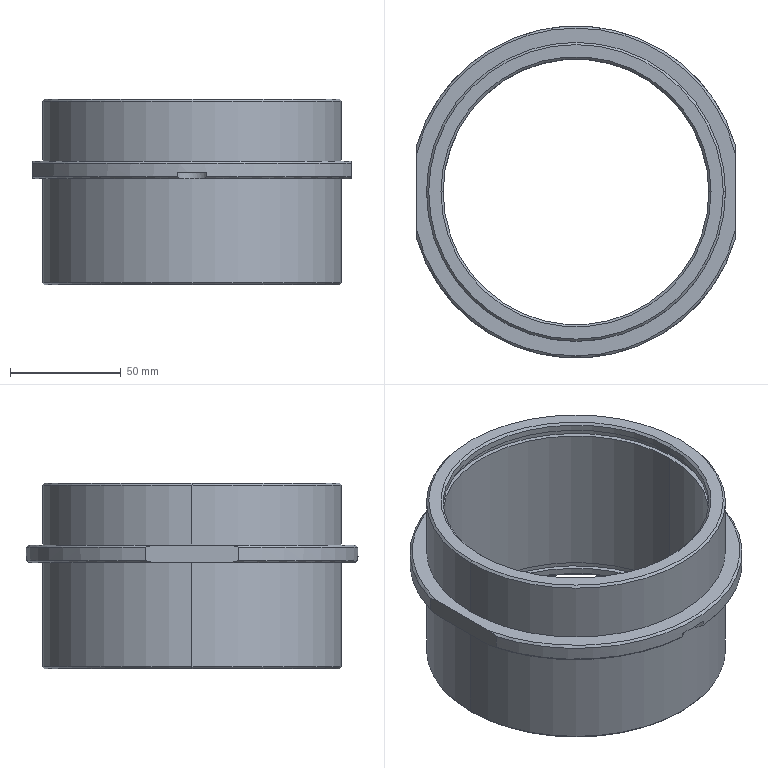Part | SolidWorks | features ICE 4, Chamfer 1, Extrusion 1, RevCut 1 | 1 solid | 44 faces | box 144 x 150 x 84 mm | volume 271588 mm3 | cylinder 18 | cone 14 | plane 12 | commonest cylinder face diameters 120 x6 124 x4 135 x4 16 x2 150 x2
STEP:
#1=CARTESIAN_POINT('',(66.5,0.,36.));
#2=VERTEX_POINT('',#1);
#3=CARTESIAN_POINT('',(-66.5,0.,36.));
#4=VERTEX_POINT('',#3);
#5=CARTESIAN_POINT('',(0.,0.,36.));
#6=DIRECTION('',(0.,0.,1.));
#7=DIRECTION('',(1.,0.,0.));
#8=AXIS2_PLACEMENT_3D('',#5,#6,#7);
#9=CIRCLE('',#8,66.5);
#10=EDGE_CURVE('',#2,#4,#9,.T.);
#11=ORIENTED_EDGE('',*,*,#10,.F.);
#12=CARTESIAN_POINT('',(67.5,0.,35.));
#13=VERTEX_POINT('',#12);
#14=CARTESIAN_POINT('',(66.5,0.,36.));
#15=DIRECTION('',(0.7071,0.,-0.7071));
#16=VECTOR('',#15,1000.);
#17=LINE('',#14,#16);
#18=EDGE_CURVE('',#2,#13,#17,.T.);
#19=ORIENTED_EDGE('',*,*,#18,.T.);
#20=CARTESIAN_POINT('',(-67.5,0.,35.));
#21=VERTEX_POINT('',#20);
#22=CARTESIAN_POINT('',(0.,0.,35.));
#23=DIRECTION('',(0.,0.,-1.));
#24=DIRECTION('',(1.,0.,0.));
#25=AXIS2_PLACEMENT_3D('',#22,#23,#24);
#26=CIRCLE('',#25,67.5);
#27=EDGE_CURVE('',#21,#13,#26,.T.);
#28=ORIENTED_EDGE('',*,*,#27,.F.);
#29=CARTESIAN_POINT('',(-66.5,0.,36.));
#30=DIRECTION('',(-0.7071,0.,-0.7071));
#31=VECTOR('',#30,1000.);
#32=LINE('',#29,#31);
#33=EDGE_CURVE('',#4,#21,#32,.T.);
#34=ORIENTED_EDGE('',*,*,#33,.F.);
#35=EDGE_LOOP('',(#11,#19,#28,#34));
#36=FACE_OUTER_BOUND('',#35,.T.);
#37=CARTESIAN_POINT('',(0.,0.,36.));
#38=DIRECTION('',(0.,0.,-1.));
#39=DIRECTION('',(-1.,0.,0.));
#40=AXIS2_PLACEMENT_3D('',#37,#38,#39);
#41=CONICAL_SURFACE('',#40,66.5,0.7854);
#42=ADVANCED_FACE('',(#36),#41,.T.);
#43=CARTESIAN_POINT('',(-60.,0.,35.));
#44=VERTEX_POINT('',#43);
#45=CARTESIAN_POINT('',(60.,0.,35.));
#46=VERTEX_POINT('',#45);
#47=CARTESIAN_POINT('',(0.,0.,35.));
#48=DIRECTION('',(0.,0.,1.));
#49=DIRECTION('',(1.,0.,0.));
#50=AXIS2_PLACEMENT_3D('',#47,#48,#49);
#51=CIRCLE('',#50,60.);
#52=EDGE_CURVE('',#44,#46,#51,.T.);
#53=ORIENTED_EDGE('',*,*,#52,.F.);
#54=CARTESIAN_POINT('',(-61.,0.,36.));
#55=VERTEX_POINT('',#54);
#56=CARTESIAN_POINT('',(-60.,0.,35.));
#57=DIRECTION('',(-0.7071,0.,0.7071));
#58=VECTOR('',#57,1000.);
#59=LINE('',#56,#58);
#60=EDGE_CURVE('',#44,#55,#59,.T.);
#61=ORIENTED_EDGE('',*,*,#60,.T.);
#62=CARTESIAN_POINT('',(61.,0.,36.));
#63=VERTEX_POINT('',#62);
#64=CARTESIAN_POINT('',(0.,0.,36.));
#65=DIRECTION('',(0.,0.,-1.));
#66=DIRECTION('',(1.,0.,0.));
#67=AXIS2_PLACEMENT_3D('',#64,#65,#66);
#68=CIRCLE('',#67,61.);
#69=EDGE_CURVE('',#63,#55,#68,.T.);
#70=ORIENTED_EDGE('',*,*,#69,.F.);
#71=CARTESIAN_POINT('',(60.,0.,35.));
#72=DIRECTION('',(0.7071,0.,0.7071));
#73=VECTOR('',#72,1000.);
#74=LINE('',#71,#73);
#75=EDGE_CURVE('',#46,#63,#74,.T.);
#76=ORIENTED_EDGE('',*,*,#75,.F.);
#77=EDGE_LOOP('',(#53,#61,#70,#76));
#78=FACE_OUTER_BOUND('',#77,.T.);
#79=CARTESIAN_POINT('',(0.,0.,35.));
#80=DIRECTION('',(0.,0.,1.));
#81=DIRECTION('',(1.,0.,0.));
#82=AXIS2_PLACEMENT_3D('',#79,#80,#81);
#83=CONICAL_SURFACE('',#82,60.,0.7854);
#84=ADVANCED_FACE('',(#78),#83,.F.);
#85=CARTESIAN_POINT('',(60.,0.,-47.));
#86=VERTEX_POINT('',#85);
#87=CARTESIAN_POINT('',(-60.,0.,-47.));
#88=VERTEX_POINT('',#87);
#89=CARTESIAN_POINT('',(0.,0.,-47.));
#90=DIRECTION('',(0.,0.,-1.));
#91=DIRECTION('',(1.,0.,0.));
#92=AXIS2_PLACEMENT_3D('',#89,#90,#91);
#93=CIRCLE('',#92,60.);
#94=EDGE_CURVE('',#86,#88,#93,.T.);
#95=ORIENTED_EDGE('',*,*,#94,.F.);
#96=CARTESIAN_POINT('',(61.,0.,-48.));
#97=VERTEX_POINT('',#96);
#98=CARTESIAN_POINT('',(61.,0.,-48.));
#99=DIRECTION('',(0.7071,0.,-0.7071));
#100=VECTOR('',#99,1000.);
#101=LINE('',#98,#100);
#102=EDGE_CURVE('',#86,#97,#101,.T.);
#103=ORIENTED_EDGE('',*,*,#102,.T.);
#104=CARTESIAN_POINT('',(-61.,0.,-48.));
#105=VERTEX_POINT('',#104);
#106=CARTESIAN_POINT('',(0.,0.,-48.));
#107=DIRECTION('',(0.,0.,1.));
#108=DIRECTION('',(1.,0.,0.));
#109=AXIS2_PLACEMENT_3D('',#106,#107,#108);
#110=CIRCLE('',#109,61.);
#111=EDGE_CURVE('',#105,#97,#110,.T.);
#112=ORIENTED_EDGE('',*,*,#111,.F.);
#113=CARTESIAN_POINT('',(-61.,0.,-48.));
#114=DIRECTION('',(-0.7071,0.,-0.7071));
#115=VECTOR('',#114,1000.);
#116=LINE('',#113,#115);
#117=EDGE_CURVE('',#88,#105,#116,.T.);
#118=ORIENTED_EDGE('',*,*,#117,.F.);
#119=EDGE_LOOP('',(#95,#103,#112,#118));
#120=FACE_OUTER_BOUND('',#119,.T.);
#121=CARTESIAN_POINT('',(0.,0.,-48.));
#122=DIRECTION('',(0.,0.,-1.));
#123=DIRECTION('',(-1.,0.,0.));
#124=AXIS2_PLACEMENT_3D('',#121,#122,#123);
#125=CONICAL_SURFACE('',#124,61.,0.7854);
#126=ADVANCED_FACE('',(#120),#125,.F.);
#127=CARTESIAN_POINT('',(-66.5,0.,-48.));
#128=VERTEX_POINT('',#127);
#129=CARTESIAN_POINT('',(66.5,0.,-48.));
#130=VERTEX_POINT('',#129);
#131=CARTESIAN_POINT('',(0.,0.,-48.));
#132=DIRECTION('',(0.,0.,-1.));
#133=DIRECTION('',(1.,0.,0.));
#134=AXIS2_PLACEMENT_3D('',#131,#132,#133);
#135=CIRCLE('',#134,66.5);
#136=EDGE_CURVE('',#128,#130,#135,.T.);
#137=ORIENTED_EDGE('',*,*,#136,.F.);
#138=CARTESIAN_POINT('',(-67.5,0.,-47.));
#139=VERTEX_POINT('',#138);
#140=CARTESIAN_POINT('',(-67.5,0.,-47.));
#141=DIRECTION('',(-0.7071,0.,0.7071));
#142=VECTOR('',#141,1000.);
#143=LINE('',#140,#142);
#144=EDGE_CURVE('',#128,#139,#143,.T.);
#145=ORIENTED_EDGE('',*,*,#144,.T.);
#146=CARTESIAN_POINT('',(67.5,0.,-47.));
#147=VERTEX_POINT('',#146);
#148=CARTESIAN_POINT('',(0.,0.,-47.));
#149=DIRECTION('',(0.,0.,1.));
#150=DIRECTION('',(1.,0.,0.));
#151=AXIS2_PLACEMENT_3D('',#148,#149,#150);
#152=CIRCLE('',#151,67.5);
#153=EDGE_CURVE('',#147,#139,#152,.T.);
#154=ORIENTED_EDGE('',*,*,#153,.F.);
#155=CARTESIAN_POINT('',(67.5,0.,-47.));
#156=DIRECTION('',(0.7071,0.,0.7071));
#157=VECTOR('',#156,1000.);
#158=LINE('',#155,#157);
#159=EDGE_CURVE('',#130,#147,#158,.T.);
#160=ORIENTED_EDGE('',*,*,#159,.F.);
#161=EDGE_LOOP('',(#137,#145,#154,#160));
#162=FACE_OUTER_BOUND('',#161,.T.);
#163=CARTESIAN_POINT('',(0.,0.,-47.));
#164=DIRECTION('',(0.,0.,1.));
#165=DIRECTION('',(1.,0.,0.));
#166=AXIS2_PLACEMENT_3D('',#163,#164,#165);
#167=CONICAL_SURFACE('',#166,67.5,0.7854);
#168=ADVANCED_FACE('',(#162),#167,.T.);
#169=CARTESIAN_POINT('',(62.,0.,32.2));
#170=VERTEX_POINT('',#169);
#171=CARTESIAN_POINT('',(-62.,0.,32.2));
#172=VERTEX_POINT('',#171);
#173=CARTESIAN_POINT('',(0.,0.,32.2));
#174=DIRECTION('',(0.,0.,-1.));
#175=DIRECTION('',(-1.,0.,0.));
#176=AXIS2_PLACEMENT_3D('',#173,#174,#175);
#177=CIRCLE('',#176,62.);
#178=EDGE_CURVE('',#170,#172,#177,.T.);
#179=ORIENTED_EDGE('',*,*,#178,.F.);
#180=CARTESIAN_POINT('',(62.,0.,29.));
#181=VERTEX_POINT('',#180);
#182=CARTESIAN_POINT('',(62.,0.,-49.991));
#183=DIRECTION('',(0.,0.,-1.));
#184=VECTOR('',#183,1000.);
#185=LINE('',#182,#184);
#186=EDGE_CURVE('',#170,#181,#185,.T.);
#187=ORIENTED_EDGE('',*,*,#186,.T.);
#188=CARTESIAN_POINT('',(-62.,0.,29.));
#189=VERTEX_POINT('',#188);
#190=CARTESIAN_POINT('',(0.,0.,29.));
#191=DIRECTION('',(0.,0.,-1.));
#192=DIRECTION('',(-1.,0.,0.));
#193=AXIS2_PLACEMENT_3D('',#190,#191,#192);
#194=CIRCLE('',#193,62.);
#195=EDGE_CURVE('',#181,#189,#194,.T.);
#196=ORIENTED_EDGE('',*,*,#195,.T.);
#197=CARTESIAN_POINT('',(-62.,0.,-49.991));
#198=DIRECTION('',(0.,0.,-1.));
#199=VECTOR('',#198,1000.);
#200=LINE('',#197,#199);
#201=EDGE_CURVE('',#172,#189,#200,.T.);
#202=ORIENTED_EDGE('',*,*,#201,.F.);
#203=EDGE_LOOP('',(#179,#187,#196,#202));
#204=FACE_OUTER_BOUND('',#203,.T.);
#205=CARTESIAN_POINT('',(0.,0.,-49.991));
#206=DIRECTION('',(0.,0.,-1.));
#207=DIRECTION('',(-1.,0.,0.));
#208=AXIS2_PLACEMENT_3D('',#205,#206,#207);
#209=CYLINDRICAL_SURFACE('',#208,62.);
#210=ADVANCED_FACE('',(#204),#209,.F.);
#211=CARTESIAN_POINT('',(60.,0.,-41.));
#212=VERTEX_POINT('',#211);
#213=CARTESIAN_POINT('',(-60.,0.,-41.));
#214=VERTEX_POINT('',#213);
#215=CARTESIAN_POINT('',(0.,0.,-41.));
#216=DIRECTION('',(0.,0.,-1.));
#217=DIRECTION('',(1.,0.,0.));
#218=AXIS2_PLACEMENT_3D('',#215,#216,#217);
#219=CIRCLE('',#218,60.);
#220=EDGE_CURVE('',#212,#214,#219,.T.);
#221=ORIENTED_EDGE('',*,*,#220,.T.);
#222=CARTESIAN_POINT('',(-60.,0.,29.));
#223=VERTEX_POINT('',#222);
#224=CARTESIAN_POINT('',(-60.,0.,-124.));
#225=DIRECTION('',(0.,0.,1.));
#226=VECTOR('',#225,1000.);
#227=LINE('',#224,#226);
#228=EDGE_CURVE('',#214,#223,#227,.T.);
#229=ORIENTED_EDGE('',*,*,#228,.T.);
#230=CARTESIAN_POINT('',(60.,0.,29.));
#231=VERTEX_POINT('',#230);
#232=CARTESIAN_POINT('',(0.,0.,29.));
#233=DIRECTION('',(0.,0.,1.));
#234=DIRECTION('',(-1.,0.,0.));
#235=AXIS2_PLACEMENT_3D('',#232,#233,#234);
#236=CIRCLE('',#235,60.);
#237=EDGE_CURVE('',#223,#231,#236,.T.);
#238=ORIENTED_EDGE('',*,*,#237,.T.);
#239=CARTESIAN_POINT('',(60.,0.,-124.));
#240=DIRECTION('',(0.,0.,1.));
#241=VECTOR('',#240,1000.);
#242=LINE('',#239,#241);
#243=EDGE_CURVE('',#212,#231,#242,.T.);
#244=ORIENTED_EDGE('',*,*,#243,.F.);
#245=EDGE_LOOP('',(#221,#229,#238,#244));
#246=FACE_OUTER_BOUND('',#245,.T.);
#247=CARTESIAN_POINT('',(0.,0.,-124.));
#248=DIRECTION('',(0.,0.,1.));
#249=DIRECTION('',(1.,0.,0.));
#250=AXIS2_PLACEMENT_3D('',#247,#248,#249);
#251=CYLINDRICAL_SURFACE('',#250,60.);
#252=ADVANCED_FACE('',(#246),#251,.F.);
#253=CARTESIAN_POINT('',(62.,0.,-41.));
#254=VERTEX_POINT('',#253);
#255=CARTESIAN_POINT('',(-62.,0.,-41.));
#256=VERTEX_POINT('',#255);
#257=CARTESIAN_POINT('',(0.,0.,-41.));
#258=DIRECTION('',(0.,0.,-1.));
#259=DIRECTION('',(-1.,0.,0.));
#260=AXIS2_PLACEMENT_3D('',#257,#258,#259);
#261=CIRCLE('',#260,62.);
#262=EDGE_CURVE('',#254,#256,#261,.T.);
#263=ORIENTED_EDGE('',*,*,#262,.F.);
#264=CARTESIAN_POINT('',(62.,0.,-44.2));
#265=VERTEX_POINT('',#264);
#266=CARTESIAN_POINT('',(62.,0.,-49.991));
#267=DIRECTION('',(0.,0.,-1.));
#268=VECTOR('',#267,1000.);
#269=LINE('',#266,#268);
#270=EDGE_CURVE('',#254,#265,#269,.T.);
#271=ORIENTED_EDGE('',*,*,#270,.T.);
#272=CARTESIAN_POINT('',(-62.,0.,-44.2));
#273=VERTEX_POINT('',#272);
#274=CARTESIAN_POINT('',(0.,0.,-44.2));
#275=DIRECTION('',(0.,0.,-1.));
#276=DIRECTION('',(-1.,0.,0.));
#277=AXIS2_PLACEMENT_3D('',#274,#275,#276);
#278=CIRCLE('',#277,62.);
#279=EDGE_CURVE('',#265,#273,#278,.T.);
#280=ORIENTED_EDGE('',*,*,#279,.T.);
#281=CARTESIAN_POINT('',(-62.,0.,-49.991));
#282=DIRECTION('',(0.,0.,-1.));
#283=VECTOR('',#282,1000.);
#284=LINE('',#281,#283);
#285=EDGE_CURVE('',#256,#273,#284,.T.);
#286=ORIENTED_EDGE('',*,*,#285,.F.);
#287=EDGE_LOOP('',(#263,#271,#280,#286));
#288=FACE_OUTER_BOUND('',#287,.T.);
#289=CARTESIAN_POINT('',(0.,0.,-49.991));
#290=DIRECTION('',(0.,0.,-1.));
#291=DIRECTION('',(-1.,0.,0.));
#292=AXIS2_PLACEMENT_3D('',#289,#290,#291);
#293=CYLINDRICAL_SURFACE('',#292,62.);
#294=ADVANCED_FACE('',(#288),#293,.F.);
#295=ORIENTED_EDGE('',*,*,#94,.T.);
#296=CARTESIAN_POINT('',(-60.,0.,-44.2));
#297=VERTEX_POINT('',#296);
#298=CARTESIAN_POINT('',(-60.,0.,-124.));
#299=DIRECTION('',(0.,0.,1.));
#300=VECTOR('',#299,1000.);
#301=LINE('',#298,#300);
#302=EDGE_CURVE('',#88,#297,#301,.T.);
#303=ORIENTED_EDGE('',*,*,#302,.T.);
#304=CARTESIAN_POINT('',(60.,0.,-44.2));
#305=VERTEX_POINT('',#304);
#306=CARTESIAN_POINT('',(0.,0.,-44.2));
#307=DIRECTION('',(0.,0.,1.));
#308=DIRECTION('',(-1.,0.,0.));
#309=AXIS2_PLACEMENT_3D('',#306,#307,#308);
#310=CIRCLE('',#309,60.);
#311=EDGE_CURVE('',#297,#305,#310,.T.);
#312=ORIENTED_EDGE('',*,*,#311,.T.);
#313=CARTESIAN_POINT('',(60.,0.,-124.));
#314=DIRECTION('',(0.,0.,1.));
#315=VECTOR('',#314,1000.);
#316=LINE('',#313,#315);
#317=EDGE_CURVE('',#86,#305,#316,.T.);
#318=ORIENTED_EDGE('',*,*,#317,.F.);
#319=EDGE_LOOP('',(#295,#303,#312,#318));
#320=FACE_OUTER_BOUND('',#319,.T.);
#321=CARTESIAN_POINT('',(0.,0.,-124.));
#322=DIRECTION('',(0.,0.,1.));
#323=DIRECTION('',(1.,0.,0.));
#324=AXIS2_PLACEMENT_3D('',#321,#322,#323);
#325=CYLINDRICAL_SURFACE('',#324,60.);
#326=ADVANCED_FACE('',(#320),#325,.F.);
#327=CARTESIAN_POINT('',(67.5,0.,8.));
#328=VERTEX_POINT('',#327);
#329=CARTESIAN_POINT('',(-67.5,0.,8.));
#330=VERTEX_POINT('',#329);
#331=CARTESIAN_POINT('',(0.,0.,8.));
#332=DIRECTION('',(0.,0.,1.));
#333=DIRECTION('',(1.,0.,0.));
#334=AXIS2_PLACEMENT_3D('',#331,#332,#333);
#335=CIRCLE('',#334,67.5);
#336=EDGE_CURVE('',#328,#330,#335,.T.);
#337=ORIENTED_EDGE('',*,*,#336,.T.);
#338=CARTESIAN_POINT('',(-67.5,0.,-48.));
#339=DIRECTION('',(0.,0.,1.));
#340=VECTOR('',#339,1000.);
#341=LINE('',#338,#340);
#342=EDGE_CURVE('',#330,#21,#341,.T.);
#343=ORIENTED_EDGE('',*,*,#342,.T.);
#344=ORIENTED_EDGE('',*,*,#27,.T.);
#345=CARTESIAN_POINT('',(67.5,0.,-48.));
#346=DIRECTION('',(0.,0.,1.));
#347=VECTOR('',#346,1000.);
#348=LINE('',#345,#347);
#349=EDGE_CURVE('',#328,#13,#348,.T.);
#350=ORIENTED_EDGE('',*,*,#349,.F.);
#351=EDGE_LOOP('',(#337,#343,#344,#350));
#352=FACE_OUTER_BOUND('',#351,.T.);
#353=CARTESIAN_POINT('',(0.,0.,-48.));
#354=DIRECTION('',(0.,0.,1.));
#355=DIRECTION('',(1.,0.,0.));
#356=AXIS2_PLACEMENT_3D('',#353,#354,#355);
#357=CYLINDRICAL_SURFACE('',#356,67.5);
#358=ADVANCED_FACE('',(#352),#357,.T.);
#359=ORIENTED_EDGE('',*,*,#153,.T.);
#360=CARTESIAN_POINT('',(-67.5,0.,0.));
#361=VERTEX_POINT('',#360);
#362=CARTESIAN_POINT('',(-67.5,0.,-48.));
#363=DIRECTION('',(0.,0.,1.));
#364=VECTOR('',#363,1000.);
#365=LINE('',#362,#364);
#366=EDGE_CURVE('',#139,#361,#365,.T.);
#367=ORIENTED_EDGE('',*,*,#366,.T.);
#368=CARTESIAN_POINT('',(67.5,0.,0.));
#369=VERTEX_POINT('',#368);
#370=CARTESIAN_POINT('',(0.,0.,0.));
#371=DIRECTION('',(0.,0.,1.));
#372=DIRECTION('',(1.,0.,0.));
#373=AXIS2_PLACEMENT_3D('',#370,#371,#372);
#374=CIRCLE('',#373,67.5);
#375=EDGE_CURVE('',#369,#361,#374,.T.);
#376=ORIENTED_EDGE('',*,*,#375,.F.);
#377=CARTESIAN_POINT('',(67.5,0.,-48.));
#378=DIRECTION('',(0.,0.,1.));
#379=VECTOR('',#378,1000.);
#380=LINE('',#377,#379);
#381=EDGE_CURVE('',#147,#369,#380,.T.);
#382=ORIENTED_EDGE('',*,*,#381,.F.);
#383=EDGE_LOOP('',(#359,#367,#376,#382));
#384=FACE_OUTER_BOUND('',#383,.T.);
#385=CARTESIAN_POINT('',(0.,0.,-48.));
#386=DIRECTION('',(0.,0.,1.));
#387=DIRECTION('',(1.,0.,0.));
#388=AXIS2_PLACEMENT_3D('',#385,#386,#387);
#389=CYLINDRICAL_SURFACE('',#388,67.5);
#390=ADVANCED_FACE('',(#384),#389,.T.);
#391=CARTESIAN_POINT('',(60.,0.,32.2));
#392=VERTEX_POINT('',#391);
#393=CARTESIAN_POINT('',(-60.,0.,32.2));
#394=VERTEX_POINT('',#393);
#395=CARTESIAN_POINT('',(0.,0.,32.2));
#396=DIRECTION('',(0.,0.,-1.));
#397=DIRECTION('',(1.,0.,0.));
#398=AXIS2_PLACEMENT_3D('',#395,#396,#397);
#399=CIRCLE('',#398,60.);
#400=EDGE_CURVE('',#392,#394,#399,.T.);
#401=ORIENTED_EDGE('',*,*,#400,.T.);
#402=CARTESIAN_POINT('',(-60.,0.,-124.));
#403=DIRECTION('',(0.,0.,1.));
#404=VECTOR('',#403,1000.);
#405=LINE('',#402,#404);
#406=EDGE_CURVE('',#394,#44,#405,.T.);
#407=ORIENTED_EDGE('',*,*,#406,.T.);
#408=ORIENTED_EDGE('',*,*,#52,.T.);
#409=CARTESIAN_POINT('',(60.,0.,-124.));
#410=DIRECTION('',(0.,0.,1.));
#411=VECTOR('',#410,1000.);
#412=LINE('',#409,#411);
#413=EDGE_CURVE('',#392,#46,#412,.T.);
#414=ORIENTED_EDGE('',*,*,#413,.F.);
#415=EDGE_LOOP('',(#401,#407,#408,#414));
#416=FACE_OUTER_BOUND('',#415,.T.);
#417=CARTESIAN_POINT('',(0.,0.,-124.));
#418=DIRECTION('',(0.,0.,1.));
#419=DIRECTION('',(1.,0.,0.));
#420=AXIS2_PLACEMENT_3D('',#417,#418,#419);
#421=CYLINDRICAL_SURFACE('',#420,60.);
#422=ADVANCED_FACE('',(#416),#421,.F.);
#423=CARTESIAN_POINT('',(6.419,74.725,3.));
#424=VERTEX_POINT('',#423);
#425=CARTESIAN_POINT('',(6.419,74.725,1.));
#426=VERTEX_POINT('',#425);
#427=CARTESIAN_POINT('',(6.419,74.725,1.5));
#428=DIRECTION('',(0.,0.,-1.));
#429=VECTOR('',#428,1000.);
#430=LINE('',#427,#429);
#431=EDGE_CURVE('',#424,#426,#430,.T.);
#432=ORIENTED_EDGE('',*,*,#431,.F.);
#433=CARTESIAN_POINT('',(-6.419,74.725,3.));
#434=VERTEX_POINT('',#433);
#435=CARTESIAN_POINT('',(0.,0.,3.));
#436=DIRECTION('',(0.,0.,1.));
#437=DIRECTION('',(1.,0.,0.));
#438=AXIS2_PLACEMENT_3D('',#435,#436,#437);
#439=CIRCLE('',#438,75.);
#440=EDGE_CURVE('',#424,#434,#439,.T.);
#441=ORIENTED_EDGE('',*,*,#440,.T.);
#442=CARTESIAN_POINT('',(-6.419,74.725,1.));
#443=VERTEX_POINT('',#442);
#444=CARTESIAN_POINT('',(-6.419,74.725,1.5));
#445=DIRECTION('',(0.,0.,1.));
#446=VECTOR('',#445,1000.);
#447=LINE('',#444,#446);
#448=EDGE_CURVE('',#443,#434,#447,.T.);
#449=ORIENTED_EDGE('',*,*,#448,.F.);
#450=CARTESIAN_POINT('',(-72.,21.,1.));
#451=VERTEX_POINT('',#450);
#452=CARTESIAN_POINT('',(0.,0.,1.));
#453=DIRECTION('',(0.,0.,1.));
#454=DIRECTION('',(1.,0.,0.));
#455=AXIS2_PLACEMENT_3D('',#452,#453,#454);
#456=CIRCLE('',#455,75.);
#457=EDGE_CURVE('',#443,#451,#456,.T.);
#458=ORIENTED_EDGE('',*,*,#457,.T.);
#459=CARTESIAN_POINT('',(-72.,21.,7.));
#460=VERTEX_POINT('',#459);
#461=CARTESIAN_POINT('',(-72.,21.,8.));
#462=DIRECTION('',(0.,0.,1.));
#463=VECTOR('',#462,1000.);
#464=LINE('',#461,#463);
#465=EDGE_CURVE('',#451,#460,#464,.T.);
#466=ORIENTED_EDGE('',*,*,#465,.T.);
#467=CARTESIAN_POINT('',(72.,21.,7.));
#468=VERTEX_POINT('',#467);
#469=CARTESIAN_POINT('',(0.,0.,7.));
#470=DIRECTION('',(0.,0.,-1.));
#471=DIRECTION('',(1.,0.,0.));
#472=AXIS2_PLACEMENT_3D('',#469,#470,#471);
#473=CIRCLE('',#472,75.);
#474=EDGE_CURVE('',#460,#468,#473,.T.);
#475=ORIENTED_EDGE('',*,*,#474,.T.);
#476=CARTESIAN_POINT('',(72.,21.,1.));
#477=VERTEX_POINT('',#476);
#478=CARTESIAN_POINT('',(72.,21.,8.));
#479=DIRECTION('',(0.,0.,-1.));
#480=VECTOR('',#479,1000.);
#481=LINE('',#478,#480);
#482=EDGE_CURVE('',#468,#477,#481,.T.);
#483=ORIENTED_EDGE('',*,*,#482,.T.);
#484=CARTESIAN_POINT('',(0.,0.,1.));
#485=DIRECTION('',(0.,0.,1.));
#486=DIRECTION('',(1.,0.,0.));
#487=AXIS2_PLACEMENT_3D('',#484,#485,#486);
#488=CIRCLE('',#487,75.);
#489=EDGE_CURVE('',#477,#426,#488,.T.);
#490=ORIENTED_EDGE('',*,*,#489,.T.);
#491=EDGE_LOOP('',(#432,#441,#449,#458,#466,#475,#483,#490));
#492=FACE_OUTER_BOUND('',#491,.T.);
#493=CARTESIAN_POINT('',(0.,0.,8.));
#494=DIRECTION('',(0.,0.,-1.));
#495=DIRECTION('',(-1.,0.,0.));
#496=AXIS2_PLACEMENT_3D('',#493,#494,#495);
#497=CYLINDRICAL_SURFACE('',#496,75.);
#498=ADVANCED_FACE('',(#492),#497,.T.);
#499=CARTESIAN_POINT('',(6.419,-74.725,1.));
#500=VERTEX_POINT('',#499);
#501=CARTESIAN_POINT('',(72.,-21.,1.));
#502=VERTEX_POINT('',#501);
#503=CARTESIAN_POINT('',(0.,0.,1.));
#504=DIRECTION('',(0.,0.,1.));
#505=DIRECTION('',(1.,0.,0.));
#506=AXIS2_PLACEMENT_3D('',#503,#504,#505);
#507=CIRCLE('',#506,75.);
#508=EDGE_CURVE('',#500,#502,#507,.T.);
#509=ORIENTED_EDGE('',*,*,#508,.F.);
#510=CARTESIAN_POINT('',(5.601,-73.788,0.));
#511=VERTEX_POINT('',#510);
#512=CARTESIAN_POINT('',(6.419,-74.725,1.));
#513=CARTESIAN_POINT('',(6.176,-74.399,0.6546));
#514=CARTESIAN_POINT('',(5.905,-74.086,0.3205));
#515=CARTESIAN_POINT('',(5.601,-73.788,0.));
#516=B_SPLINE_CURVE_WITH_KNOTS('',3,(#512,#513,#514,#515),.UNSPECIFIED.,.F.,.F.,(4,4),(0.000000308,0.001596),.UNSPECIFIED.);
#517=EDGE_CURVE('',#500,#511,#516,.T.);
#518=ORIENTED_EDGE('',*,*,#517,.T.);
#519=CARTESIAN_POINT('',(72.,-17.088,0.));
#520=VERTEX_POINT('',#519);
#521=CARTESIAN_POINT('',(0.,0.,0.));
#522=DIRECTION('',(0.,0.,-1.));
#523=DIRECTION('',(1.,0.,0.));
#524=AXIS2_PLACEMENT_3D('',#521,#522,#523);
#525=CIRCLE('',#524,74.);
#526=EDGE_CURVE('',#520,#511,#525,.T.);
#527=ORIENTED_EDGE('',*,*,#526,.F.);
#528=CARTESIAN_POINT('',(72.,-21.,1.));
#529=CARTESIAN_POINT('',(72.,-19.706,0.6378));
#530=CARTESIAN_POINT('',(72.,-18.403,0.3036));
#531=CARTESIAN_POINT('',(72.,-17.088,0.));
#532=B_SPLINE_CURVE_WITH_KNOTS('',3,(#528,#529,#530,#531),.UNSPECIFIED.,.F.,.F.,(4,4),(0.1572,0.1612),.UNSPECIFIED.);
#533=EDGE_CURVE('',#502,#520,#532,.T.);
#534=ORIENTED_EDGE('',*,*,#533,.F.);
#535=EDGE_LOOP('',(#509,#518,#527,#534));
#536=FACE_OUTER_BOUND('',#535,.T.);
#537=CARTESIAN_POINT('',(0.,0.,1.));
#538=DIRECTION('',(0.,0.,1.));
#539=DIRECTION('',(1.,0.,0.));
#540=AXIS2_PLACEMENT_3D('',#537,#538,#539);
#541=CONICAL_SURFACE('',#540,75.,0.7854);
#542=ADVANCED_FACE('',(#536),#541,.T.);
#543=CARTESIAN_POINT('',(-5.601,-73.788,0.));
#544=VERTEX_POINT('',#543);
#545=CARTESIAN_POINT('',(-72.,-17.088,0.));
#546=VERTEX_POINT('',#545);
#547=CARTESIAN_POINT('',(0.,0.,0.));
#548=DIRECTION('',(0.,0.,-1.));
#549=DIRECTION('',(1.,0.,0.));
#550=AXIS2_PLACEMENT_3D('',#547,#548,#549);
#551=CIRCLE('',#550,74.);
#552=EDGE_CURVE('',#544,#546,#551,.T.);
#553=ORIENTED_EDGE('',*,*,#552,.F.);
#554=CARTESIAN_POINT('',(-6.419,-74.725,1.));
#555=VERTEX_POINT('',#554);
#556=CARTESIAN_POINT('',(-5.601,-73.788,0.));
#557=CARTESIAN_POINT('',(-5.905,-74.086,0.3205));
#558=CARTESIAN_POINT('',(-6.176,-74.399,0.6546));
#559=CARTESIAN_POINT('',(-6.419,-74.725,1.));
#560=B_SPLINE_CURVE_WITH_KNOTS('',3,(#556,#557,#558,#559),.UNSPECIFIED.,.F.,.F.,(4,4),(0.000000332,0.001596),.UNSPECIFIED.);
#561=EDGE_CURVE('',#544,#555,#560,.T.);
#562=ORIENTED_EDGE('',*,*,#561,.T.);
#563=CARTESIAN_POINT('',(-72.,-21.,1.));
#564=VERTEX_POINT('',#563);
#565=CARTESIAN_POINT('',(0.,0.,1.));
#566=DIRECTION('',(0.,0.,1.));
#567=DIRECTION('',(1.,0.,0.));
#568=AXIS2_PLACEMENT_3D('',#565,#566,#567);
#569=CIRCLE('',#568,75.);
#570=EDGE_CURVE('',#564,#555,#569,.T.);
#571=ORIENTED_EDGE('',*,*,#570,.F.);
#572=CARTESIAN_POINT('',(-72.,-17.088,0.));
#573=CARTESIAN_POINT('',(-72.,-18.402,0.3035));
#574=CARTESIAN_POINT('',(-72.,-19.706,0.6376));
#575=CARTESIAN_POINT('',(-72.,-21.,1.));
#576=B_SPLINE_CURVE_WITH_KNOTS('',3,(#572,#573,#574,#575),.UNSPECIFIED.,.F.,.F.,(4,4),(0.1956,0.1997),.UNSPECIFIED.);
#577=EDGE_CURVE('',#546,#564,#576,.T.);
#578=ORIENTED_EDGE('',*,*,#577,.F.);
#579=EDGE_LOOP('',(#553,#562,#571,#578));
#580=FACE_OUTER_BOUND('',#579,.T.);
#581=CARTESIAN_POINT('',(0.,0.,1.));
#582=DIRECTION('',(0.,0.,1.));
#583=DIRECTION('',(1.,0.,0.));
#584=AXIS2_PLACEMENT_3D('',#581,#582,#583);
#585=CONICAL_SURFACE('',#584,75.,0.7854);
#586=ADVANCED_FACE('',(#580),#585,.T.);
#587=CARTESIAN_POINT('',(-6.419,-74.725,3.));
#588=VERTEX_POINT('',#587);
#589=CARTESIAN_POINT('',(-6.419,-74.725,1.5));
#590=DIRECTION('',(0.,0.,-1.));
#591=VECTOR('',#590,1000.);
#592=LINE('',#589,#591);
#593=EDGE_CURVE('',#588,#555,#592,.T.);
#594=ORIENTED_EDGE('',*,*,#593,.F.);
#595=CARTESIAN_POINT('',(6.419,-74.725,3.));
#596=VERTEX_POINT('',#595);
#597=CARTESIAN_POINT('',(0.,0.,3.));
#598=DIRECTION('',(0.,0.,1.));
#599=DIRECTION('',(1.,0.,0.));
#600=AXIS2_PLACEMENT_3D('',#597,#598,#599);
#601=CIRCLE('',#600,75.);
#602=EDGE_CURVE('',#588,#596,#601,.T.);
#603=ORIENTED_EDGE('',*,*,#602,.T.);
#604=CARTESIAN_POINT('',(6.419,-74.725,1.5));
#605=DIRECTION('',(0.,0.,1.));
#606=VECTOR('',#605,1000.);
#607=LINE('',#604,#606);
#608=EDGE_CURVE('',#500,#596,#607,.T.);
#609=ORIENTED_EDGE('',*,*,#608,.F.);
#610=ORIENTED_EDGE('',*,*,#508,.T.);
#611=CARTESIAN_POINT('',(72.,-21.,7.));
#612=VERTEX_POINT('',#611);
#613=CARTESIAN_POINT('',(72.,-21.,8.));
#614=DIRECTION('',(0.,0.,1.));
#615=VECTOR('',#614,1000.);
#616=LINE('',#613,#615);
#617=EDGE_CURVE('',#502,#612,#616,.T.);
#618=ORIENTED_EDGE('',*,*,#617,.T.);
#619=CARTESIAN_POINT('',(-72.,-21.,7.));
#620=VERTEX_POINT('',#619);
#621=CARTESIAN_POINT('',(0.,0.,7.));
#622=DIRECTION('',(0.,0.,-1.));
#623=DIRECTION('',(1.,0.,0.));
#624=AXIS2_PLACEMENT_3D('',#621,#622,#623);
#625=CIRCLE('',#624,75.);
#626=EDGE_CURVE('',#612,#620,#625,.T.);
#627=ORIENTED_EDGE('',*,*,#626,.T.);
#628=CARTESIAN_POINT('',(-72.,-21.,8.));
#629=DIRECTION('',(0.,0.,-1.));
#630=VECTOR('',#629,1000.);
#631=LINE('',#628,#630);
#632=EDGE_CURVE('',#620,#564,#631,.T.);
#633=ORIENTED_EDGE('',*,*,#632,.T.);
#634=ORIENTED_EDGE('',*,*,#570,.T.);
#635=EDGE_LOOP('',(#594,#603,#609,#610,#618,#627,#633,#634));
#636=FACE_OUTER_BOUND('',#635,.T.);
#637=CARTESIAN_POINT('',(0.,0.,8.));
#638=DIRECTION('',(0.,0.,-1.));
#639=DIRECTION('',(-1.,0.,0.));
#640=AXIS2_PLACEMENT_3D('',#637,#638,#639);
#641=CYLINDRICAL_SURFACE('',#640,75.);
#642=ADVANCED_FACE('',(#636),#641,.T.);
#643=ORIENTED_EDGE('',*,*,#457,.F.);
#644=CARTESIAN_POINT('',(-5.601,73.788,0.));
#645=VERTEX_POINT('',#644);
#646=CARTESIAN_POINT('',(-6.419,74.725,1.));
#647=CARTESIAN_POINT('',(-6.176,74.399,0.6546));
#648=CARTESIAN_POINT('',(-5.905,74.086,0.3205));
#649=CARTESIAN_POINT('',(-5.601,73.788,0.));
#650=B_SPLINE_CURVE_WITH_KNOTS('',3,(#646,#647,#648,#649),.UNSPECIFIED.,.F.,.F.,(4,4),(0.000000308,0.001596),.UNSPECIFIED.);
#651=EDGE_CURVE('',#443,#645,#650,.T.);
#652=ORIENTED_EDGE('',*,*,#651,.T.);
#653=CARTESIAN_POINT('',(-72.,17.088,0.));
#654=VERTEX_POINT('',#653);
#655=CARTESIAN_POINT('',(0.,0.,0.));
#656=DIRECTION('',(0.,0.,-1.));
#657=DIRECTION('',(1.,0.,0.));
#658=AXIS2_PLACEMENT_3D('',#655,#656,#657);
#659=CIRCLE('',#658,74.);
#660=EDGE_CURVE('',#654,#645,#659,.T.);
#661=ORIENTED_EDGE('',*,*,#660,.F.);
#662=CARTESIAN_POINT('',(-72.,21.,1.));
#663=CARTESIAN_POINT('',(-72.,19.706,0.6378));
#664=CARTESIAN_POINT('',(-72.,18.403,0.3036));
#665=CARTESIAN_POINT('',(-72.,17.088,0.));
#666=B_SPLINE_CURVE_WITH_KNOTS('',3,(#662,#663,#664,#665),.UNSPECIFIED.,.F.,.F.,(4,4),(0.1572,0.1612),.UNSPECIFIED.);
#667=EDGE_CURVE('',#451,#654,#666,.T.);
#668=ORIENTED_EDGE('',*,*,#667,.F.);
#669=EDGE_LOOP('',(#643,#652,#661,#668));
#670=FACE_OUTER_BOUND('',#669,.T.);
#671=CARTESIAN_POINT('',(0.,0.,1.));
#672=DIRECTION('',(0.,0.,1.));
#673=DIRECTION('',(1.,0.,0.));
#674=AXIS2_PLACEMENT_3D('',#671,#672,#673);
#675=CONICAL_SURFACE('',#674,75.,0.7854);
#676=ADVANCED_FACE('',(#670),#675,.T.);
#677=CARTESIAN_POINT('',(5.601,73.788,0.));
#678=VERTEX_POINT('',#677);
#679=CARTESIAN_POINT('',(72.,17.088,0.));
#680=VERTEX_POINT('',#679);
#681=CARTESIAN_POINT('',(0.,0.,0.));
#682=DIRECTION('',(0.,0.,-1.));
#683=DIRECTION('',(1.,0.,0.));
#684=AXIS2_PLACEMENT_3D('',#681,#682,#683);
#685=CIRCLE('',#684,74.);
#686=EDGE_CURVE('',#678,#680,#685,.T.);
#687=ORIENTED_EDGE('',*,*,#686,.F.);
#688=CARTESIAN_POINT('',(5.601,73.788,0.));
#689=CARTESIAN_POINT('',(5.905,74.086,0.3205));
#690=CARTESIAN_POINT('',(6.176,74.399,0.6546));
#691=CARTESIAN_POINT('',(6.419,74.725,1.));
#692=B_SPLINE_CURVE_WITH_KNOTS('',3,(#688,#689,#690,#691),.UNSPECIFIED.,.F.,.F.,(4,4),(0.000000332,0.001596),.UNSPECIFIED.);
#693=EDGE_CURVE('',#678,#426,#692,.T.);
#694=ORIENTED_EDGE('',*,*,#693,.T.);
#695=ORIENTED_EDGE('',*,*,#489,.F.);
#696=CARTESIAN_POINT('',(72.,17.088,0.));
#697=CARTESIAN_POINT('',(72.,18.402,0.3035));
#698=CARTESIAN_POINT('',(72.,19.706,0.6376));
#699=CARTESIAN_POINT('',(72.,21.,1.));
#700=B_SPLINE_CURVE_WITH_KNOTS('',3,(#696,#697,#698,#699),.UNSPECIFIED.,.F.,.F.,(4,4),(0.1956,0.1997),.UNSPECIFIED.);
#701=EDGE_CURVE('',#680,#477,#700,.T.);
#702=ORIENTED_EDGE('',*,*,#701,.F.);
#703=EDGE_LOOP('',(#687,#694,#695,#702));
#704=FACE_OUTER_BOUND('',#703,.T.);
#705=CARTESIAN_POINT('',(0.,0.,1.));
#706=DIRECTION('',(0.,0.,1.));
#707=DIRECTION('',(1.,0.,0.));
#708=AXIS2_PLACEMENT_3D('',#705,#706,#707);
#709=CONICAL_SURFACE('',#708,75.,0.7854);
#710=ADVANCED_FACE('',(#704),#709,.T.);
#711=CARTESIAN_POINT('',(72.,17.088,8.));
#712=VERTEX_POINT('',#711);
#713=CARTESIAN_POINT('',(72.,21.,7.));
#714=CARTESIAN_POINT('',(72.,19.706,7.362));
#715=CARTESIAN_POINT('',(72.,18.403,7.696));
#716=CARTESIAN_POINT('',(72.,17.088,8.));
#717=B_SPLINE_CURVE_WITH_KNOTS('',3,(#713,#714,#715,#716),.UNSPECIFIED.,.F.,.F.,(4,4),(0.1572,0.1612),.UNSPECIFIED.);
#718=EDGE_CURVE('',#468,#712,#717,.T.);
#719=ORIENTED_EDGE('',*,*,#718,.F.);
#720=ORIENTED_EDGE('',*,*,#474,.F.);
#721=CARTESIAN_POINT('',(-72.,17.088,8.));
#722=VERTEX_POINT('',#721);
#723=CARTESIAN_POINT('',(-72.,17.088,8.));
#724=CARTESIAN_POINT('',(-72.,18.402,7.697));
#725=CARTESIAN_POINT('',(-72.,19.706,7.362));
#726=CARTESIAN_POINT('',(-72.,21.,7.));
#727=B_SPLINE_CURVE_WITH_KNOTS('',3,(#723,#724,#725,#726),.UNSPECIFIED.,.F.,.F.,(4,4),(0.1956,0.1997),.UNSPECIFIED.);
#728=EDGE_CURVE('',#722,#460,#727,.T.);
#729=ORIENTED_EDGE('',*,*,#728,.F.);
#730=CARTESIAN_POINT('',(0.,0.,8.));
#731=DIRECTION('',(0.,0.,1.));
#732=DIRECTION('',(1.,0.,0.));
#733=AXIS2_PLACEMENT_3D('',#730,#731,#732);
#734=CIRCLE('',#733,74.);
#735=EDGE_CURVE('',#712,#722,#734,.T.);
#736=ORIENTED_EDGE('',*,*,#735,.F.);
#737=EDGE_LOOP('',(#719,#720,#729,#736));
#738=FACE_OUTER_BOUND('',#737,.T.);
#739=CARTESIAN_POINT('',(0.,0.,8.));
#740=DIRECTION('',(0.,0.,-1.));
#741=DIRECTION('',(-1.,0.,0.));
#742=AXIS2_PLACEMENT_3D('',#739,#740,#741);
#743=CONICAL_SURFACE('',#742,74.,0.7854);
#744=ADVANCED_FACE('',(#738),#743,.T.);
#745=ORIENTED_EDGE('',*,*,#406,.F.);
#746=CARTESIAN_POINT('',(0.,0.,32.2));
#747=DIRECTION('',(0.,0.,-1.));
#748=DIRECTION('',(1.,0.,0.));
#749=AXIS2_PLACEMENT_3D('',#746,#747,#748);
#750=CIRCLE('',#749,60.);
#751=EDGE_CURVE('',#394,#392,#750,.T.);
#752=ORIENTED_EDGE('',*,*,#751,.T.);
#753=ORIENTED_EDGE('',*,*,#413,.T.);
#754=CARTESIAN_POINT('',(0.,0.,35.));
#755=DIRECTION('',(0.,0.,1.));
#756=DIRECTION('',(1.,0.,0.));
#757=AXIS2_PLACEMENT_3D('',#754,#755,#756);
#758=CIRCLE('',#757,60.);
#759=EDGE_CURVE('',#46,#44,#758,.T.);
#760=ORIENTED_EDGE('',*,*,#759,.T.);
#761=EDGE_LOOP('',(#745,#752,#753,#760));
#762=FACE_OUTER_BOUND('',#761,.T.);
#763=CARTESIAN_POINT('',(0.,0.,-124.));
#764=DIRECTION('',(0.,0.,1.));
#765=DIRECTION('',(1.,0.,0.));
#766=AXIS2_PLACEMENT_3D('',#763,#764,#765);
#767=CYLINDRICAL_SURFACE('',#766,60.);
#768=ADVANCED_FACE('',(#762),#767,.F.);
#769=CARTESIAN_POINT('',(72.,-17.088,8.));
#770=VERTEX_POINT('',#769);
#771=CARTESIAN_POINT('',(72.,0.,8.));
#772=DIRECTION('',(0.,-1.,0.));
#773=VECTOR('',#772,1000.);
#774=LINE('',#771,#773);
#775=EDGE_CURVE('',#712,#770,#774,.T.);
#776=ORIENTED_EDGE('',*,*,#775,.F.);
#777=ORIENTED_EDGE('',*,*,#735,.T.);
#778=CARTESIAN_POINT('',(-72.,-17.088,8.));
#779=VERTEX_POINT('',#778);
#780=CARTESIAN_POINT('',(-72.,0.,8.));
#781=DIRECTION('',(0.,1.,0.));
#782=VECTOR('',#781,1000.);
#783=LINE('',#780,#782);
#784=EDGE_CURVE('',#779,#722,#783,.T.);
#785=ORIENTED_EDGE('',*,*,#784,.F.);
#786=CARTESIAN_POINT('',(0.,0.,8.));
#787=DIRECTION('',(0.,0.,1.));
#788=DIRECTION('',(1.,0.,0.));
#789=AXIS2_PLACEMENT_3D('',#786,#787,#788);
#790=CIRCLE('',#789,74.);
#791=EDGE_CURVE('',#779,#770,#790,.T.);
#792=ORIENTED_EDGE('',*,*,#791,.T.);
#793=EDGE_LOOP('',(#776,#777,#785,#792));
#794=FACE_OUTER_BOUND('',#793,.T.);
#795=ORIENTED_EDGE('',*,*,#336,.F.);
#796=CARTESIAN_POINT('',(0.,0.,8.));
#797=DIRECTION('',(0.,0.,1.));
#798=DIRECTION('',(1.,0.,0.));
#799=AXIS2_PLACEMENT_3D('',#796,#797,#798);
#800=CIRCLE('',#799,67.5);
#801=EDGE_CURVE('',#330,#328,#800,.T.);
#802=ORIENTED_EDGE('',*,*,#801,.F.);
#803=EDGE_LOOP('',(#795,#802));
#804=FACE_BOUND('',#803,.T.);
#805=CARTESIAN_POINT('',(0.,0.,8.));
#806=DIRECTION('',(0.,0.,1.));
#807=DIRECTION('',(1.,0.,0.));
#808=AXIS2_PLACEMENT_3D('',#805,#806,#807);
#809=PLANE('',#808);
#810=ADVANCED_FACE('',(#794,#804),#809,.T.);
#811=CARTESIAN_POINT('',(0.,79.5,0.));
#812=DIRECTION('',(0.,0.,1.));
#813=DIRECTION('',(1.,0.,0.));
#814=AXIS2_PLACEMENT_3D('',#811,#812,#813);
#815=CIRCLE('',#814,8.);
#816=EDGE_CURVE('',#645,#678,#815,.T.);
#817=ORIENTED_EDGE('',*,*,#816,.T.);
#818=ORIENTED_EDGE('',*,*,#686,.T.);
#819=CARTESIAN_POINT('',(72.,75.,0.));
#820=DIRECTION('',(0.,1.,0.));
#821=VECTOR('',#820,1000.);
#822=LINE('',#819,#821);
#823=EDGE_CURVE('',#520,#680,#822,.T.);
#824=ORIENTED_EDGE('',*,*,#823,.F.);
#825=ORIENTED_EDGE('',*,*,#526,.T.);
#826=CARTESIAN_POINT('',(0.,-79.5,0.));
#827=DIRECTION('',(0.,0.,1.));
#828=DIRECTION('',(1.,0.,0.));
#829=AXIS2_PLACEMENT_3D('',#826,#827,#828);
#830=CIRCLE('',#829,8.);
#831=EDGE_CURVE('',#511,#544,#830,.T.);
#832=ORIENTED_EDGE('',*,*,#831,.T.);
#833=ORIENTED_EDGE('',*,*,#552,.T.);
#834=CARTESIAN_POINT('',(-72.,75.,0.));
#835=DIRECTION('',(0.,-1.,0.));
#836=VECTOR('',#835,1000.);
#837=LINE('',#834,#836);
#838=EDGE_CURVE('',#654,#546,#837,.T.);
#839=ORIENTED_EDGE('',*,*,#838,.F.);
#840=ORIENTED_EDGE('',*,*,#660,.T.);
#841=EDGE_LOOP('',(#817,#818,#824,#825,#832,#833,#839,#840));
#842=FACE_OUTER_BOUND('',#841,.T.);
#843=ORIENTED_EDGE('',*,*,#375,.T.);
#844=CARTESIAN_POINT('',(0.,0.,0.));
#845=DIRECTION('',(0.,0.,1.));
#846=DIRECTION('',(1.,0.,0.));
#847=AXIS2_PLACEMENT_3D('',#844,#845,#846);
#848=CIRCLE('',#847,67.5);
#849=EDGE_CURVE('',#361,#369,#848,.T.);
#850=ORIENTED_EDGE('',*,*,#849,.T.);
#851=EDGE_LOOP('',(#843,#850));
#852=FACE_BOUND('',#851,.T.);
#853=CARTESIAN_POINT('',(0.,0.,0.));
#854=DIRECTION('',(0.,0.,1.));
#855=DIRECTION('',(1.,0.,0.));
#856=AXIS2_PLACEMENT_3D('',#853,#854,#855);
#857=PLANE('',#856);
#858=ADVANCED_FACE('',(#842,#852),#857,.F.);
#859=CARTESIAN_POINT('',(0.,0.,-48.));
#860=DIRECTION('',(0.,0.,-1.));
#861=DIRECTION('',(1.,0.,0.));
#862=AXIS2_PLACEMENT_3D('',#859,#860,#861);
#863=CIRCLE('',#862,66.5);
#864=EDGE_CURVE('',#130,#128,#863,.T.);
#865=ORIENTED_EDGE('',*,*,#864,.T.);
#866=ORIENTED_EDGE('',*,*,#136,.T.);
#867=EDGE_LOOP('',(#865,#866));
#868=FACE_OUTER_BOUND('',#867,.T.);
#869=ORIENTED_EDGE('',*,*,#111,.T.);
#870=CARTESIAN_POINT('',(0.,0.,-48.));
#871=DIRECTION('',(0.,0.,1.));
#872=DIRECTION('',(1.,0.,0.));
#873=AXIS2_PLACEMENT_3D('',#870,#871,#872);
#874=CIRCLE('',#873,61.);
#875=EDGE_CURVE('',#97,#105,#874,.T.);
#876=ORIENTED_EDGE('',*,*,#875,.T.);
#877=EDGE_LOOP('',(#869,#876));
#878=FACE_BOUND('',#877,.T.);
#879=CARTESIAN_POINT('',(0.,0.,-48.));
#880=DIRECTION('',(0.,0.,1.));
#881=DIRECTION('',(1.,0.,0.));
#882=AXIS2_PLACEMENT_3D('',#879,#880,#881);
#883=PLANE('',#882);
#884=ADVANCED_FACE('',(#868,#878),#883,.F.);
#885=ORIENTED_EDGE('',*,*,#366,.F.);
#886=CARTESIAN_POINT('',(0.,0.,-47.));
#887=DIRECTION('',(0.,0.,1.));
#888=DIRECTION('',(1.,0.,0.));
#889=AXIS2_PLACEMENT_3D('',#886,#887,#888);
#890=CIRCLE('',#889,67.5);
#891=EDGE_CURVE('',#139,#147,#890,.T.);
#892=ORIENTED_EDGE('',*,*,#891,.T.);
#893=ORIENTED_EDGE('',*,*,#381,.T.);
#894=ORIENTED_EDGE('',*,*,#849,.F.);
#895=EDGE_LOOP('',(#885,#892,#893,#894));
#896=FACE_OUTER_BOUND('',#895,.T.);
#897=CARTESIAN_POINT('',(0.,0.,-48.));
#898=DIRECTION('',(0.,0.,1.));
#899=DIRECTION('',(1.,0.,0.));
#900=AXIS2_PLACEMENT_3D('',#897,#898,#899);
#901=CYLINDRICAL_SURFACE('',#900,67.5);
#902=ADVANCED_FACE('',(#896),#901,.T.);
#903=ORIENTED_EDGE('',*,*,#342,.F.);
#904=ORIENTED_EDGE('',*,*,#801,.T.);
#905=ORIENTED_EDGE('',*,*,#349,.T.);
#906=CARTESIAN_POINT('',(0.,0.,35.));
#907=DIRECTION('',(0.,0.,-1.));
#908=DIRECTION('',(1.,0.,0.));
#909=AXIS2_PLACEMENT_3D('',#906,#907,#908);
#910=CIRCLE('',#909,67.5);
#911=EDGE_CURVE('',#13,#21,#910,.T.);
#912=ORIENTED_EDGE('',*,*,#911,.T.);
#913=EDGE_LOOP('',(#903,#904,#905,#912));
#914=FACE_OUTER_BOUND('',#913,.T.);
#915=CARTESIAN_POINT('',(0.,0.,-48.));
#916=DIRECTION('',(0.,0.,1.));
#917=DIRECTION('',(1.,0.,0.));
#918=AXIS2_PLACEMENT_3D('',#915,#916,#917);
#919=CYLINDRICAL_SURFACE('',#918,67.5);
#920=ADVANCED_FACE('',(#914),#919,.T.);
#921=ORIENTED_EDGE('',*,*,#69,.T.);
#922=CARTESIAN_POINT('',(0.,0.,36.));
#923=DIRECTION('',(0.,0.,-1.));
#924=DIRECTION('',(1.,0.,0.));
#925=AXIS2_PLACEMENT_3D('',#922,#923,#924);
#926=CIRCLE('',#925,61.);
#927=EDGE_CURVE('',#55,#63,#926,.T.);
#928=ORIENTED_EDGE('',*,*,#927,.T.);
#929=EDGE_LOOP('',(#921,#928));
#930=FACE_BOUND('',#929,.T.);
#931=CARTESIAN_POINT('',(0.,0.,36.));
#932=DIRECTION('',(0.,0.,1.));
#933=DIRECTION('',(1.,0.,0.));
#934=AXIS2_PLACEMENT_3D('',#931,#932,#933);
#935=CIRCLE('',#934,66.5);
#936=EDGE_CURVE('',#4,#2,#935,.T.);
#937=ORIENTED_EDGE('',*,*,#936,.T.);
#938=ORIENTED_EDGE('',*,*,#10,.T.);
#939=EDGE_LOOP('',(#937,#938));
#940=FACE_OUTER_BOUND('',#939,.T.);
#941=CARTESIAN_POINT('',(0.,0.,36.));
#942=DIRECTION('',(0.,0.,1.));
#943=DIRECTION('',(1.,0.,0.));
#944=AXIS2_PLACEMENT_3D('',#941,#942,#943);
#945=PLANE('',#944);
#946=ADVANCED_FACE('',(#930,#940),#945,.T.);
#947=ORIENTED_EDGE('',*,*,#302,.F.);
#948=CARTESIAN_POINT('',(0.,0.,-47.));
#949=DIRECTION('',(0.,0.,-1.));
#950=DIRECTION('',(1.,0.,0.));
#951=AXIS2_PLACEMENT_3D('',#948,#949,#950);
#952=CIRCLE('',#951,60.);
#953=EDGE_CURVE('',#88,#86,#952,.T.);
#954=ORIENTED_EDGE('',*,*,#953,.T.);
#955=ORIENTED_EDGE('',*,*,#317,.T.);
#956=CARTESIAN_POINT('',(0.,0.,-44.2));
#957=DIRECTION('',(0.,0.,1.));
#958=DIRECTION('',(-1.,0.,0.));
#959=AXIS2_PLACEMENT_3D('',#956,#957,#958);
#960=CIRCLE('',#959,60.);
#961=EDGE_CURVE('',#305,#297,#960,.T.);
#962=ORIENTED_EDGE('',*,*,#961,.T.);
#963=EDGE_LOOP('',(#947,#954,#955,#962));
#964=FACE_OUTER_BOUND('',#963,.T.);
#965=CARTESIAN_POINT('',(0.,0.,-124.));
#966=DIRECTION('',(0.,0.,1.));
#967=DIRECTION('',(1.,0.,0.));
#968=AXIS2_PLACEMENT_3D('',#965,#966,#967);
#969=CYLINDRICAL_SURFACE('',#968,60.);
#970=ADVANCED_FACE('',(#964),#969,.F.);
#971=CARTESIAN_POINT('',(0.,0.,-41.));
#972=DIRECTION('',(0.,0.,-1.));
#973=DIRECTION('',(-1.,0.,0.));
#974=AXIS2_PLACEMENT_3D('',#971,#972,#973);
#975=CIRCLE('',#974,62.);
#976=EDGE_CURVE('',#256,#254,#975,.T.);
#977=ORIENTED_EDGE('',*,*,#976,.T.);
#978=ORIENTED_EDGE('',*,*,#262,.T.);
#979=EDGE_LOOP('',(#977,#978));
#980=FACE_OUTER_BOUND('',#979,.T.);
#981=ORIENTED_EDGE('',*,*,#220,.F.);
#982=CARTESIAN_POINT('',(0.,0.,-41.));
#983=DIRECTION('',(0.,0.,-1.));
#984=DIRECTION('',(1.,0.,0.));
#985=AXIS2_PLACEMENT_3D('',#982,#983,#984);
#986=CIRCLE('',#985,60.);
#987=EDGE_CURVE('',#214,#212,#986,.T.);
#988=ORIENTED_EDGE('',*,*,#987,.F.);
#989=EDGE_LOOP('',(#981,#988));
#990=FACE_BOUND('',#989,.T.);
#991=CARTESIAN_POINT('',(-62.,0.,-41.));
#992=DIRECTION('',(0.,0.,1.));
#993=DIRECTION('',(1.,0.,0.));
#994=AXIS2_PLACEMENT_3D('',#991,#992,#993);
#995=PLANE('',#994);
#996=ADVANCED_FACE('',(#980,#990),#995,.F.);
#997=CARTESIAN_POINT('',(0.,0.,-44.2));
#998=DIRECTION('',(0.,0.,-1.));
#999=DIRECTION('',(-1.,0.,0.));
#1000=AXIS2_PLACEMENT_3D('',#997,#998,#999);
#1001=CIRCLE('',#1000,62.);
#1002=EDGE_CURVE('',#273,#265,#1001,.T.);
#1003=ORIENTED_EDGE('',*,*,#1002,.F.);
#1004=ORIENTED_EDGE('',*,*,#279,.F.);
#1005=EDGE_LOOP('',(#1003,#1004));
#1006=FACE_OUTER_BOUND('',#1005,.T.);
#1007=ORIENTED_EDGE('',*,*,#961,.F.);
#1008=ORIENTED_EDGE('',*,*,#311,.F.);
#1009=EDGE_LOOP('',(#1007,#1008));
#1010=FACE_BOUND('',#1009,.T.);
#1011=CARTESIAN_POINT('',(-62.,0.,-44.2));
#1012=DIRECTION('',(0.,0.,-1.));
#1013=DIRECTION('',(-1.,0.,0.));
#1014=AXIS2_PLACEMENT_3D('',#1011,#1012,#1013);
#1015=PLANE('',#1014);
#1016=ADVANCED_FACE('',(#1006,#1010),#1015,.F.);
#1017=ORIENTED_EDGE('',*,*,#270,.F.);
#1018=ORIENTED_EDGE('',*,*,#976,.F.);
#1019=ORIENTED_EDGE('',*,*,#285,.T.);
#1020=ORIENTED_EDGE('',*,*,#1002,.T.);
#1021=EDGE_LOOP('',(#1017,#1018,#1019,#1020));
#1022=FACE_OUTER_BOUND('',#1021,.T.);
#1023=CARTESIAN_POINT('',(0.,0.,-49.991));
#1024=DIRECTION('',(0.,0.,-1.));
#1025=DIRECTION('',(-1.,0.,0.));
#1026=AXIS2_PLACEMENT_3D('',#1023,#1024,#1025);
#1027=CYLINDRICAL_SURFACE('',#1026,62.);
#1028=ADVANCED_FACE('',(#1022),#1027,.F.);
#1029=ORIENTED_EDGE('',*,*,#228,.F.);
#1030=ORIENTED_EDGE('',*,*,#987,.T.);
#1031=ORIENTED_EDGE('',*,*,#243,.T.);
#1032=CARTESIAN_POINT('',(0.,0.,29.));
#1033=DIRECTION('',(0.,0.,1.));
#1034=DIRECTION('',(-1.,0.,0.));
#1035=AXIS2_PLACEMENT_3D('',#1032,#1033,#1034);
#1036=CIRCLE('',#1035,60.);
#1037=EDGE_CURVE('',#231,#223,#1036,.T.);
#1038=ORIENTED_EDGE('',*,*,#1037,.T.);
#1039=EDGE_LOOP('',(#1029,#1030,#1031,#1038));
#1040=FACE_OUTER_BOUND('',#1039,.T.);
#1041=CARTESIAN_POINT('',(0.,0.,-124.));
#1042=DIRECTION('',(0.,0.,1.));
#1043=DIRECTION('',(1.,0.,0.));
#1044=AXIS2_PLACEMENT_3D('',#1041,#1042,#1043);
#1045=CYLINDRICAL_SURFACE('',#1044,60.);
#1046=ADVANCED_FACE('',(#1040),#1045,.F.);
#1047=CARTESIAN_POINT('',(0.,0.,32.2));
#1048=DIRECTION('',(0.,0.,-1.));
#1049=DIRECTION('',(-1.,0.,0.));
#1050=AXIS2_PLACEMENT_3D('',#1047,#1048,#1049);
#1051=CIRCLE('',#1050,62.);
#1052=EDGE_CURVE('',#172,#170,#1051,.T.);
#1053=ORIENTED_EDGE('',*,*,#1052,.T.);
#1054=ORIENTED_EDGE('',*,*,#178,.T.);
#1055=EDGE_LOOP('',(#1053,#1054));
#1056=FACE_OUTER_BOUND('',#1055,.T.);
#1057=ORIENTED_EDGE('',*,*,#400,.F.);
#1058=ORIENTED_EDGE('',*,*,#751,.F.);
#1059=EDGE_LOOP('',(#1057,#1058));
#1060=FACE_BOUND('',#1059,.T.);
#1061=CARTESIAN_POINT('',(-56.802,0.,32.2));
#1062=DIRECTION('',(0.,0.,1.));
#1063=DIRECTION('',(1.,0.,0.));
#1064=AXIS2_PLACEMENT_3D('',#1061,#1062,#1063);
#1065=PLANE('',#1064);
#1066=ADVANCED_FACE('',(#1056,#1060),#1065,.F.);
#1067=CARTESIAN_POINT('',(0.,0.,29.));
#1068=DIRECTION('',(0.,0.,-1.));
#1069=DIRECTION('',(-1.,0.,0.));
#1070=AXIS2_PLACEMENT_3D('',#1067,#1068,#1069);
#1071=CIRCLE('',#1070,62.);
#1072=EDGE_CURVE('',#189,#181,#1071,.T.);
#1073=ORIENTED_EDGE('',*,*,#1072,.F.);
#1074=ORIENTED_EDGE('',*,*,#195,.F.);
#1075=EDGE_LOOP('',(#1073,#1074));
#1076=FACE_OUTER_BOUND('',#1075,.T.);
#1077=ORIENTED_EDGE('',*,*,#1037,.F.);
#1078=ORIENTED_EDGE('',*,*,#237,.F.);
#1079=EDGE_LOOP('',(#1077,#1078));
#1080=FACE_BOUND('',#1079,.T.);
#1081=CARTESIAN_POINT('',(-56.802,0.,29.));
#1082=DIRECTION('',(0.,0.,-1.));
#1083=DIRECTION('',(-1.,0.,0.));
#1084=AXIS2_PLACEMENT_3D('',#1081,#1082,#1083);
#1085=PLANE('',#1084);
#1086=ADVANCED_FACE('',(#1076,#1080),#1085,.F.);
#1087=ORIENTED_EDGE('',*,*,#186,.F.);
#1088=ORIENTED_EDGE('',*,*,#1052,.F.);
#1089=ORIENTED_EDGE('',*,*,#201,.T.);
#1090=ORIENTED_EDGE('',*,*,#1072,.T.);
#1091=EDGE_LOOP('',(#1087,#1088,#1089,#1090));
#1092=FACE_OUTER_BOUND('',#1091,.T.);
#1093=CARTESIAN_POINT('',(0.,0.,-49.991));
#1094=DIRECTION('',(0.,0.,-1.));
#1095=DIRECTION('',(-1.,0.,0.));
#1096=AXIS2_PLACEMENT_3D('',#1093,#1094,#1095);
#1097=CYLINDRICAL_SURFACE('',#1096,62.);
#1098=ADVANCED_FACE('',(#1092),#1097,.F.);
#1099=ORIENTED_EDGE('',*,*,#144,.F.);
#1100=ORIENTED_EDGE('',*,*,#864,.F.);
#1101=ORIENTED_EDGE('',*,*,#159,.T.);
#1102=ORIENTED_EDGE('',*,*,#891,.F.);
#1103=EDGE_LOOP('',(#1099,#1100,#1101,#1102));
#1104=FACE_OUTER_BOUND('',#1103,.T.);
#1105=CARTESIAN_POINT('',(0.,0.,-47.));
#1106=DIRECTION('',(0.,0.,1.));
#1107=DIRECTION('',(1.,0.,0.));
#1108=AXIS2_PLACEMENT_3D('',#1105,#1106,#1107);
#1109=CONICAL_SURFACE('',#1108,67.5,0.7854);
#1110=ADVANCED_FACE('',(#1104),#1109,.T.);
#1111=CARTESIAN_POINT('',(72.,-17.088,8.));
#1112=CARTESIAN_POINT('',(72.,-18.402,7.697));
#1113=CARTESIAN_POINT('',(72.,-19.706,7.362));
#1114=CARTESIAN_POINT('',(72.,-21.,7.));
#1115=B_SPLINE_CURVE_WITH_KNOTS('',3,(#1111,#1112,#1113,#1114),.UNSPECIFIED.,.F.,.F.,(4,4),(0.1956,0.1997),.UNSPECIFIED.);
#1116=EDGE_CURVE('',#770,#612,#1115,.T.);
#1117=ORIENTED_EDGE('',*,*,#1116,.F.);
#1118=ORIENTED_EDGE('',*,*,#791,.F.);
#1119=CARTESIAN_POINT('',(-72.,-21.,7.));
#1120=CARTESIAN_POINT('',(-72.,-19.706,7.362));
#1121=CARTESIAN_POINT('',(-72.,-18.403,7.696));
#1122=CARTESIAN_POINT('',(-72.,-17.088,8.));
#1123=B_SPLINE_CURVE_WITH_KNOTS('',3,(#1119,#1120,#1121,#1122),.UNSPECIFIED.,.F.,.F.,(4,4),(0.1572,0.1612),.UNSPECIFIED.);
#1124=EDGE_CURVE('',#620,#779,#1123,.T.);
#1125=ORIENTED_EDGE('',*,*,#1124,.F.);
#1126=ORIENTED_EDGE('',*,*,#626,.F.);
#1127=EDGE_LOOP('',(#1117,#1118,#1125,#1126));
#1128=FACE_OUTER_BOUND('',#1127,.T.);
#1129=CARTESIAN_POINT('',(0.,0.,8.));
#1130=DIRECTION('',(0.,0.,-1.));
#1131=DIRECTION('',(-1.,0.,0.));
#1132=AXIS2_PLACEMENT_3D('',#1129,#1130,#1131);
#1133=CONICAL_SURFACE('',#1132,74.,0.7854);
#1134=ADVANCED_FACE('',(#1128),#1133,.T.);
#1135=ORIENTED_EDGE('',*,*,#102,.F.);
#1136=ORIENTED_EDGE('',*,*,#953,.F.);
#1137=ORIENTED_EDGE('',*,*,#117,.T.);
#1138=ORIENTED_EDGE('',*,*,#875,.F.);
#1139=EDGE_LOOP('',(#1135,#1136,#1137,#1138));
#1140=FACE_OUTER_BOUND('',#1139,.T.);
#1141=CARTESIAN_POINT('',(0.,0.,-48.));
#1142=DIRECTION('',(0.,0.,-1.));
#1143=DIRECTION('',(-1.,0.,0.));
#1144=AXIS2_PLACEMENT_3D('',#1141,#1142,#1143);
#1145=CONICAL_SURFACE('',#1144,61.,0.7854);
#1146=ADVANCED_FACE('',(#1140),#1145,.F.);
#1147=ORIENTED_EDGE('',*,*,#60,.F.);
#1148=ORIENTED_EDGE('',*,*,#759,.F.);
#1149=ORIENTED_EDGE('',*,*,#75,.T.);
#1150=ORIENTED_EDGE('',*,*,#927,.F.);
#1151=EDGE_LOOP('',(#1147,#1148,#1149,#1150));
#1152=FACE_OUTER_BOUND('',#1151,.T.);
#1153=CARTESIAN_POINT('',(0.,0.,35.));
#1154=DIRECTION('',(0.,0.,1.));
#1155=DIRECTION('',(1.,0.,0.));
#1156=AXIS2_PLACEMENT_3D('',#1153,#1154,#1155);
#1157=CONICAL_SURFACE('',#1156,60.,0.7854);
#1158=ADVANCED_FACE('',(#1152),#1157,.F.);
#1159=ORIENTED_EDGE('',*,*,#18,.F.);
#1160=ORIENTED_EDGE('',*,*,#936,.F.);
#1161=ORIENTED_EDGE('',*,*,#33,.T.);
#1162=ORIENTED_EDGE('',*,*,#911,.F.);
#1163=EDGE_LOOP('',(#1159,#1160,#1161,#1162));
#1164=FACE_OUTER_BOUND('',#1163,.T.);
#1165=CARTESIAN_POINT('',(0.,0.,36.));
#1166=DIRECTION('',(0.,0.,-1.));
#1167=DIRECTION('',(-1.,0.,0.));
#1168=AXIS2_PLACEMENT_3D('',#1165,#1166,#1167);
#1169=CONICAL_SURFACE('',#1168,66.5,0.7854);
#1170=ADVANCED_FACE('',(#1164),#1169,.T.);
#1171=ORIENTED_EDGE('',*,*,#577,.T.);
#1172=ORIENTED_EDGE('',*,*,#632,.F.);
#1173=ORIENTED_EDGE('',*,*,#1124,.T.);
#1174=ORIENTED_EDGE('',*,*,#784,.T.);
#1175=ORIENTED_EDGE('',*,*,#728,.T.);
#1176=ORIENTED_EDGE('',*,*,#465,.F.);
#1177=ORIENTED_EDGE('',*,*,#667,.T.);
#1178=ORIENTED_EDGE('',*,*,#838,.T.);
#1179=EDGE_LOOP('',(#1171,#1172,#1173,#1174,#1175,#1176,#1177,#1178));
#1180=FACE_OUTER_BOUND('',#1179,.T.);
#1181=CARTESIAN_POINT('',(-72.,75.,72.));
#1182=DIRECTION('',(1.,0.,0.));
#1183=DIRECTION('',(0.,1.,0.));
#1184=AXIS2_PLACEMENT_3D('',#1181,#1182,#1183);
#1185=PLANE('',#1184);
#1186=ADVANCED_FACE('',(#1180),#1185,.F.);
#1187=ORIENTED_EDGE('',*,*,#701,.T.);
#1188=ORIENTED_EDGE('',*,*,#482,.F.);
#1189=ORIENTED_EDGE('',*,*,#718,.T.);
#1190=ORIENTED_EDGE('',*,*,#775,.T.);
#1191=ORIENTED_EDGE('',*,*,#1116,.T.);
#1192=ORIENTED_EDGE('',*,*,#617,.F.);
#1193=ORIENTED_EDGE('',*,*,#533,.T.);
#1194=ORIENTED_EDGE('',*,*,#823,.T.);
#1195=EDGE_LOOP('',(#1187,#1188,#1189,#1190,#1191,#1192,#1193,#1194));
#1196=FACE_OUTER_BOUND('',#1195,.T.);
#1197=CARTESIAN_POINT('',(72.,75.,72.));
#1198=DIRECTION('',(-1.,0.,0.));
#1199=DIRECTION('',(0.,-1.,0.));
#1200=AXIS2_PLACEMENT_3D('',#1197,#1198,#1199);
#1201=PLANE('',#1200);
#1202=ADVANCED_FACE('',(#1196),#1201,.F.);
#1203=CARTESIAN_POINT('',(0.,79.5,3.));
#1204=DIRECTION('',(0.,0.,1.));
#1205=DIRECTION('',(1.,0.,0.));
#1206=AXIS2_PLACEMENT_3D('',#1203,#1204,#1205);
#1207=CIRCLE('',#1206,8.);
#1208=EDGE_CURVE('',#434,#424,#1207,.T.);
#1209=ORIENTED_EDGE('',*,*,#1208,.F.);
#1210=ORIENTED_EDGE('',*,*,#440,.F.);
#1211=EDGE_LOOP('',(#1209,#1210));
#1212=FACE_OUTER_BOUND('',#1211,.T.);
#1213=CARTESIAN_POINT('',(0.,79.5,3.));
#1214=DIRECTION('',(0.,0.,1.));
#1215=DIRECTION('',(1.,0.,0.));
#1216=AXIS2_PLACEMENT_3D('',#1213,#1214,#1215);
#1217=PLANE('',#1216);
#1218=ADVANCED_FACE('',(#1212),#1217,.F.);
#1219=ORIENTED_EDGE('',*,*,#448,.T.);
#1220=ORIENTED_EDGE('',*,*,#1208,.T.);
#1221=ORIENTED_EDGE('',*,*,#431,.T.);
#1222=ORIENTED_EDGE('',*,*,#693,.F.);
#1223=ORIENTED_EDGE('',*,*,#816,.F.);
#1224=ORIENTED_EDGE('',*,*,#651,.F.);
#1225=EDGE_LOOP('',(#1219,#1220,#1221,#1222,#1223,#1224));
#1226=FACE_OUTER_BOUND('',#1225,.T.);
#1227=CARTESIAN_POINT('',(0.,79.5,3.));
#1228=DIRECTION('',(0.,0.,-1.));
#1229=DIRECTION('',(-1.,0.,0.));
#1230=AXIS2_PLACEMENT_3D('',#1227,#1228,#1229);
#1231=CYLINDRICAL_SURFACE('',#1230,8.);
#1232=ADVANCED_FACE('',(#1226),#1231,.F.);
#1233=CARTESIAN_POINT('',(0.,-79.5,3.));
#1234=DIRECTION('',(0.,0.,1.));
#1235=DIRECTION('',(1.,0.,0.));
#1236=AXIS2_PLACEMENT_3D('',#1233,#1234,#1235);
#1237=CIRCLE('',#1236,8.);
#1238=EDGE_CURVE('',#596,#588,#1237,.T.);
#1239=ORIENTED_EDGE('',*,*,#1238,.F.);
#1240=ORIENTED_EDGE('',*,*,#602,.F.);
#1241=EDGE_LOOP('',(#1239,#1240));
#1242=FACE_OUTER_BOUND('',#1241,.T.);
#1243=CARTESIAN_POINT('',(0.,-79.5,3.));
#1244=DIRECTION('',(0.,0.,1.));
#1245=DIRECTION('',(1.,0.,0.));
#1246=AXIS2_PLACEMENT_3D('',#1243,#1244,#1245);
#1247=PLANE('',#1246);
#1248=ADVANCED_FACE('',(#1242),#1247,.F.);
#1249=ORIENTED_EDGE('',*,*,#831,.F.);
#1250=ORIENTED_EDGE('',*,*,#517,.F.);
#1251=ORIENTED_EDGE('',*,*,#608,.T.);
#1252=ORIENTED_EDGE('',*,*,#1238,.T.);
#1253=ORIENTED_EDGE('',*,*,#593,.T.);
#1254=ORIENTED_EDGE('',*,*,#561,.F.);
#1255=EDGE_LOOP('',(#1249,#1250,#1251,#1252,#1253,#1254));
#1256=FACE_OUTER_BOUND('',#1255,.T.);
#1257=CARTESIAN_POINT('',(0.,-79.5,3.));
#1258=DIRECTION('',(0.,0.,-1.));
#1259=DIRECTION('',(-1.,0.,0.));
#1260=AXIS2_PLACEMENT_3D('',#1257,#1258,#1259);
#1261=CYLINDRICAL_SURFACE('',#1260,8.);
#1262=ADVANCED_FACE('',(#1256),#1261,.F.);
#1263=CLOSED_SHELL('',(#42,#84,#126,#168,#210,#252,#294,#326,#358,#390,#422,#498,#542,#586,#642,#676,#710,#744,#768,#810,#858,#884,#902,#920,#946,#970,#996,#1016,#1028,#1046,#1066,#1086,#1098,#1110,#1134,#1146,#1158,#1170,#1186,#1202,#1218,#1232,#1248,#1262));
#1264=MANIFOLD_SOLID_BREP('',#1263);
#1265=CARTESIAN_POINT('',(0.,0.,0.));
#1266=DIRECTION('',(0.,0.,1.));
#1267=DIRECTION('',(1.,0.,0.));
#1268=AXIS2_PLACEMENT_3D('',#1265,#1266,#1267);
#1269=(LENGTH_UNIT()NAMED_UNIT(*)SI_UNIT(.MILLI.,.METRE.));
#1270=UNCERTAINTY_MEASURE_WITH_UNIT(LENGTH_MEASURE(0.00001),#1269,'','');
#1271=(NAMED_UNIT(*)PLANE_ANGLE_UNIT()SI_UNIT($,.RADIAN.));
#1272=(NAMED_UNIT(*)SI_UNIT($,.STERADIAN.)SOLID_ANGLE_UNIT());
#1273=(GEOMETRIC_REPRESENTATION_CONTEXT(3)GLOBAL_UNCERTAINTY_ASSIGNED_CONTEXT((#1270))GLOBAL_UNIT_ASSIGNED_CONTEXT((#1269,#1271,#1272))REPRESENTATION_CONTEXT('',''));
#1274=ADVANCED_BREP_SHAPE_REPRESENTATION('',(#1264,#1268),#1273);